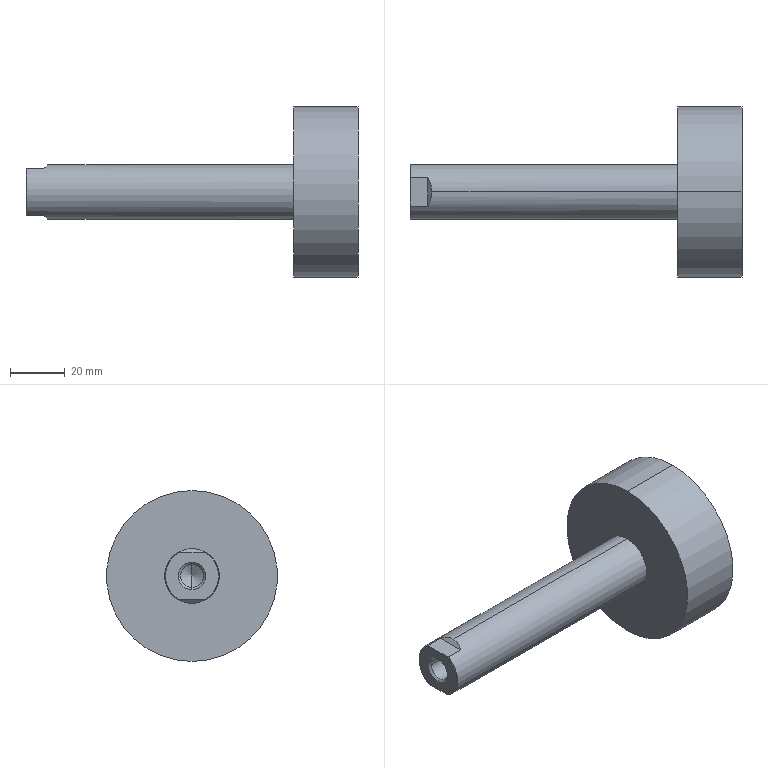Part | SolidWorks | features BaseBody 1 | 1 solid | 19 faces | box 121.5 x 62.5 x 62.5 mm | volume 101686 mm3 | plane 7 | cylinder 6 | cone 6 | commonest cylinder face diameters 8.376 x2 20 x2 62.5 x2
STEP:
#1=CARTESIAN_POINT('',(-1.5,5.268,8.5));
#2=VERTEX_POINT('',#1);
#3=CARTESIAN_POINT('',(0.,0.,10.));
#4=VERTEX_POINT('',#3);
#5=CARTESIAN_POINT('',(-1.5,5.268,8.5));
#6=CARTESIAN_POINT('',(-0.5131,3.675,9.487));
#7=CARTESIAN_POINT('',(0.,1.873,10.));
#8=CARTESIAN_POINT('',(0.,0.,10.));
#9=(BOUNDED_CURVE()B_SPLINE_CURVE(3,(#5,#6,#7,#8),.UNSPECIFIED.,.F.,.T.)B_SPLINE_CURVE_WITH_KNOTS((4,4),(5.728,6.283),.UNSPECIFIED.)CURVE()GEOMETRIC_REPRESENTATION_ITEM()RATIONAL_B_SPLINE_CURVE((1.,0.9745,0.9745,1.))REPRESENTATION_ITEM(''));
#10=EDGE_CURVE('',#2,#4,#9,.T.);
#11=ORIENTED_EDGE('',*,*,#10,.T.);
#12=CARTESIAN_POINT('',(90.,0.,10.));
#13=VERTEX_POINT('',#12);
#14=CARTESIAN_POINT('',(0.,0.,10.));
#15=DIRECTION('',(1.,0.,0.));
#16=VECTOR('',#15,1000.);
#17=LINE('',#14,#16);
#18=EDGE_CURVE('',#4,#13,#17,.T.);
#19=ORIENTED_EDGE('',*,*,#18,.T.);
#20=CARTESIAN_POINT('',(90.,0.,-10.));
#21=VERTEX_POINT('',#20);
#22=CARTESIAN_POINT('',(90.,0.,0.));
#23=DIRECTION('',(-1.,0.,0.));
#24=DIRECTION('',(0.,0.,-1.));
#25=AXIS2_PLACEMENT_3D('',#22,#23,#24);
#26=CIRCLE('',#25,10.);
#27=EDGE_CURVE('',#13,#21,#26,.T.);
#28=ORIENTED_EDGE('',*,*,#27,.T.);
#29=CARTESIAN_POINT('',(0.,0.,-10.));
#30=VERTEX_POINT('',#29);
#31=CARTESIAN_POINT('',(0.,0.,-10.));
#32=DIRECTION('',(1.,0.,0.));
#33=VECTOR('',#32,1000.);
#34=LINE('',#31,#33);
#35=EDGE_CURVE('',#30,#21,#34,.T.);
#36=ORIENTED_EDGE('',*,*,#35,.F.);
#37=CARTESIAN_POINT('',(-1.5,5.268,-8.5));
#38=VERTEX_POINT('',#37);
#39=CARTESIAN_POINT('',(0.,0.,-10.));
#40=CARTESIAN_POINT('',(0.,1.873,-10.));
#41=CARTESIAN_POINT('',(-0.5131,3.675,-9.487));
#42=CARTESIAN_POINT('',(-1.5,5.268,-8.5));
#43=(BOUNDED_CURVE()B_SPLINE_CURVE(3,(#39,#40,#41,#42),.UNSPECIFIED.,.F.,.T.)B_SPLINE_CURVE_WITH_KNOTS((4,4),(0.,0.5548),.UNSPECIFIED.)CURVE()GEOMETRIC_REPRESENTATION_ITEM()RATIONAL_B_SPLINE_CURVE((1.,0.9745,0.9745,1.))REPRESENTATION_ITEM(''));
#44=EDGE_CURVE('',#30,#38,#43,.T.);
#45=ORIENTED_EDGE('',*,*,#44,.T.);
#46=CARTESIAN_POINT('',(-7.75,5.268,-8.5));
#47=VERTEX_POINT('',#46);
#48=CARTESIAN_POINT('',(0.,5.268,-8.5));
#49=DIRECTION('',(-1.,0.,0.));
#50=VECTOR('',#49,1000.);
#51=LINE('',#48,#50);
#52=EDGE_CURVE('',#38,#47,#51,.T.);
#53=ORIENTED_EDGE('',*,*,#52,.T.);
#54=CARTESIAN_POINT('',(-7.75,5.268,8.5));
#55=VERTEX_POINT('',#54);
#56=CARTESIAN_POINT('',(-7.75,0.,0.));
#57=DIRECTION('',(1.,0.,0.));
#58=DIRECTION('',(0.,0.,-1.));
#59=AXIS2_PLACEMENT_3D('',#56,#57,#58);
#60=CIRCLE('',#59,10.);
#61=EDGE_CURVE('',#47,#55,#60,.T.);
#62=ORIENTED_EDGE('',*,*,#61,.T.);
#63=CARTESIAN_POINT('',(0.,5.268,8.5));
#64=DIRECTION('',(1.,0.,0.));
#65=VECTOR('',#64,1000.);
#66=LINE('',#63,#65);
#67=EDGE_CURVE('',#55,#2,#66,.T.);
#68=ORIENTED_EDGE('',*,*,#67,.T.);
#69=EDGE_LOOP('',(#11,#19,#28,#36,#45,#53,#62,#68));
#70=FACE_OUTER_BOUND('',#69,.T.);
#71=CARTESIAN_POINT('',(0.,0.,0.));
#72=DIRECTION('',(1.,0.,0.));
#73=DIRECTION('',(0.,0.,-1.));
#74=AXIS2_PLACEMENT_3D('',#71,#72,#73);
#75=CYLINDRICAL_SURFACE('',#74,10.);
#76=ADVANCED_FACE('',(#70),#75,.T.);
#77=CARTESIAN_POINT('',(90.,0.,-31.25));
#78=VERTEX_POINT('',#77);
#79=CARTESIAN_POINT('',(90.,0.,31.25));
#80=VERTEX_POINT('',#79);
#81=CARTESIAN_POINT('',(90.,0.,0.));
#82=DIRECTION('',(1.,0.,0.));
#83=DIRECTION('',(0.,0.,-1.));
#84=AXIS2_PLACEMENT_3D('',#81,#82,#83);
#85=CIRCLE('',#84,31.25);
#86=EDGE_CURVE('',#78,#80,#85,.T.);
#87=ORIENTED_EDGE('',*,*,#86,.T.);
#88=CARTESIAN_POINT('',(113.5,0.,31.25));
#89=VERTEX_POINT('',#88);
#90=CARTESIAN_POINT('',(113.5,0.,31.25));
#91=DIRECTION('',(1.,0.,0.));
#92=VECTOR('',#91,1000.);
#93=LINE('',#90,#92);
#94=EDGE_CURVE('',#80,#89,#93,.T.);
#95=ORIENTED_EDGE('',*,*,#94,.T.);
#96=CARTESIAN_POINT('',(113.5,0.,-31.25));
#97=VERTEX_POINT('',#96);
#98=CARTESIAN_POINT('',(113.5,0.,0.));
#99=DIRECTION('',(-1.,0.,0.));
#100=DIRECTION('',(0.,0.,-1.));
#101=AXIS2_PLACEMENT_3D('',#98,#99,#100);
#102=CIRCLE('',#101,31.25);
#103=EDGE_CURVE('',#89,#97,#102,.T.);
#104=ORIENTED_EDGE('',*,*,#103,.T.);
#105=CARTESIAN_POINT('',(113.5,0.,-31.25));
#106=DIRECTION('',(1.,0.,0.));
#107=VECTOR('',#106,1000.);
#108=LINE('',#105,#107);
#109=EDGE_CURVE('',#78,#97,#108,.T.);
#110=ORIENTED_EDGE('',*,*,#109,.F.);
#111=EDGE_LOOP('',(#87,#95,#104,#110));
#112=FACE_OUTER_BOUND('',#111,.T.);
#113=CARTESIAN_POINT('',(113.5,0.,0.));
#114=DIRECTION('',(1.,0.,0.));
#115=DIRECTION('',(0.,0.,-1.));
#116=AXIS2_PLACEMENT_3D('',#113,#114,#115);
#117=CYLINDRICAL_SURFACE('',#116,31.25);
#118=ADVANCED_FACE('',(#112),#117,.T.);
#119=CARTESIAN_POINT('',(-7.188,0.,-4.188));
#120=VERTEX_POINT('',#119);
#121=CARTESIAN_POINT('',(-7.188,-4.188,0.));
#122=VERTEX_POINT('',#121);
#123=CARTESIAN_POINT('',(-7.188,0.,0.));
#124=DIRECTION('',(-1.,0.,0.));
#125=DIRECTION('',(0.,-1.,0.));
#126=AXIS2_PLACEMENT_3D('',#123,#124,#125);
#127=CIRCLE('',#126,4.188);
#128=EDGE_CURVE('',#120,#122,#127,.T.);
#129=ORIENTED_EDGE('',*,*,#128,.F.);
#130=CARTESIAN_POINT('',(-8.,0.,-5.));
#131=VERTEX_POINT('',#130);
#132=CARTESIAN_POINT('',(-8.,0.,-5.));
#133=DIRECTION('',(-0.7071,0.,-0.7071));
#134=VECTOR('',#133,1000.);
#135=LINE('',#132,#134);
#136=EDGE_CURVE('',#120,#131,#135,.T.);
#137=ORIENTED_EDGE('',*,*,#136,.T.);
#138=CARTESIAN_POINT('',(-8.,0.,5.));
#139=VERTEX_POINT('',#138);
#140=CARTESIAN_POINT('',(-8.,0.,0.));
#141=DIRECTION('',(-1.,0.,0.));
#142=DIRECTION('',(0.,0.,1.));
#143=AXIS2_PLACEMENT_3D('',#140,#141,#142);
#144=CIRCLE('',#143,5.);
#145=EDGE_CURVE('',#131,#139,#144,.T.);
#146=ORIENTED_EDGE('',*,*,#145,.T.);
#147=CARTESIAN_POINT('',(-7.188,0.,4.188));
#148=VERTEX_POINT('',#147);
#149=CARTESIAN_POINT('',(-8.,0.,5.));
#150=DIRECTION('',(-0.7071,0.,0.7071));
#151=VECTOR('',#150,1000.);
#152=LINE('',#149,#151);
#153=EDGE_CURVE('',#148,#139,#152,.T.);
#154=ORIENTED_EDGE('',*,*,#153,.F.);
#155=CARTESIAN_POINT('',(-7.188,0.,0.));
#156=DIRECTION('',(-1.,0.,0.));
#157=DIRECTION('',(0.,-1.,0.));
#158=AXIS2_PLACEMENT_3D('',#155,#156,#157);
#159=CIRCLE('',#158,4.188);
#160=EDGE_CURVE('',#122,#148,#159,.T.);
#161=ORIENTED_EDGE('',*,*,#160,.F.);
#162=EDGE_LOOP('',(#129,#137,#146,#154,#161));
#163=FACE_OUTER_BOUND('',#162,.T.);
#164=CARTESIAN_POINT('',(-8.,0.,0.));
#165=DIRECTION('',(-1.,0.,0.));
#166=DIRECTION('',(0.,0.,1.));
#167=AXIS2_PLACEMENT_3D('',#164,#165,#166);
#168=CONICAL_SURFACE('',#167,5.,0.7854);
#169=ADVANCED_FACE('',(#163),#168,.F.);
#170=CARTESIAN_POINT('',(-7.188,4.188,0.));
#171=VERTEX_POINT('',#170);
#172=CARTESIAN_POINT('',(-7.188,0.,0.));
#173=DIRECTION('',(-1.,0.,0.));
#174=DIRECTION('',(0.,-1.,0.));
#175=AXIS2_PLACEMENT_3D('',#172,#173,#174);
#176=CIRCLE('',#175,4.188);
#177=EDGE_CURVE('',#171,#120,#176,.T.);
#178=ORIENTED_EDGE('',*,*,#177,.T.);
#179=ORIENTED_EDGE('',*,*,#128,.T.);
#180=CARTESIAN_POINT('',(10.,-4.188,0.));
#181=VERTEX_POINT('',#180);
#182=CARTESIAN_POINT('',(12.418,-4.188,0.));
#183=DIRECTION('',(1.,0.,0.));
#184=VECTOR('',#183,1000.);
#185=LINE('',#182,#184);
#186=EDGE_CURVE('',#122,#181,#185,.T.);
#187=ORIENTED_EDGE('',*,*,#186,.T.);
#188=CARTESIAN_POINT('',(10.,0.,-4.188));
#189=VERTEX_POINT('',#188);
#190=CARTESIAN_POINT('',(10.,0.,0.));
#191=DIRECTION('',(-1.,0.,0.));
#192=DIRECTION('',(0.,1.,0.));
#193=AXIS2_PLACEMENT_3D('',#190,#191,#192);
#194=CIRCLE('',#193,4.188);
#195=EDGE_CURVE('',#189,#181,#194,.T.);
#196=ORIENTED_EDGE('',*,*,#195,.F.);
#197=CARTESIAN_POINT('',(10.,4.188,0.));
#198=VERTEX_POINT('',#197);
#199=CARTESIAN_POINT('',(10.,0.,0.));
#200=DIRECTION('',(-1.,0.,0.));
#201=DIRECTION('',(0.,1.,0.));
#202=AXIS2_PLACEMENT_3D('',#199,#200,#201);
#203=CIRCLE('',#202,4.188);
#204=EDGE_CURVE('',#198,#189,#203,.T.);
#205=ORIENTED_EDGE('',*,*,#204,.F.);
#206=CARTESIAN_POINT('',(12.418,4.188,0.));
#207=DIRECTION('',(1.,0.,0.));
#208=VECTOR('',#207,1000.);
#209=LINE('',#206,#208);
#210=EDGE_CURVE('',#171,#198,#209,.T.);
#211=ORIENTED_EDGE('',*,*,#210,.F.);
#212=EDGE_LOOP('',(#178,#179,#187,#196,#205,#211));
#213=FACE_OUTER_BOUND('',#212,.T.);
#214=CARTESIAN_POINT('',(12.418,0.,0.));
#215=DIRECTION('',(1.,0.,0.));
#216=DIRECTION('',(0.,1.,0.));
#217=AXIS2_PLACEMENT_3D('',#214,#215,#216);
#218=CYLINDRICAL_SURFACE('',#217,4.188);
#219=ADVANCED_FACE('',(#213),#218,.F.);
#220=CARTESIAN_POINT('',(12.418,0.,0.));
#221=VERTEX_POINT('',#220);
#222=CARTESIAN_POINT('',(10.,0.,4.188));
#223=VERTEX_POINT('',#222);
#224=CARTESIAN_POINT('',(10.,0.,4.188));
#225=DIRECTION('',(-0.5,0.,0.866));
#226=VECTOR('',#225,1000.);
#227=LINE('',#224,#226);
#228=EDGE_CURVE('',#221,#223,#227,.T.);
#229=ORIENTED_EDGE('',*,*,#228,.F.);
#230=CARTESIAN_POINT('',(10.,0.,-4.188));
#231=DIRECTION('',(-0.5,0.,-0.866));
#232=VECTOR('',#231,1000.);
#233=LINE('',#230,#232);
#234=EDGE_CURVE('',#221,#189,#233,.T.);
#235=ORIENTED_EDGE('',*,*,#234,.T.);
#236=ORIENTED_EDGE('',*,*,#195,.T.);
#237=CARTESIAN_POINT('',(10.,0.,0.));
#238=DIRECTION('',(-1.,0.,0.));
#239=DIRECTION('',(0.,1.,0.));
#240=AXIS2_PLACEMENT_3D('',#237,#238,#239);
#241=CIRCLE('',#240,4.188);
#242=EDGE_CURVE('',#181,#223,#241,.T.);
#243=ORIENTED_EDGE('',*,*,#242,.T.);
#244=EDGE_LOOP('',(#229,#235,#236,#243));
#245=FACE_OUTER_BOUND('',#244,.T.);
#246=CARTESIAN_POINT('',(10.,0.,0.));
#247=DIRECTION('',(-1.,0.,0.));
#248=DIRECTION('',(0.,0.,1.));
#249=AXIS2_PLACEMENT_3D('',#246,#247,#248);
#250=CONICAL_SURFACE('',#249,4.188,1.047);
#251=ADVANCED_FACE('',(#245),#250,.F.);
#252=ORIENTED_EDGE('',*,*,#18,.F.);
#253=CARTESIAN_POINT('',(-1.5,-5.268,8.5));
#254=VERTEX_POINT('',#253);
#255=CARTESIAN_POINT('',(0.,0.,10.));
#256=CARTESIAN_POINT('',(0.,-1.873,10.));
#257=CARTESIAN_POINT('',(-0.5131,-3.675,9.487));
#258=CARTESIAN_POINT('',(-1.5,-5.268,8.5));
#259=(BOUNDED_CURVE()B_SPLINE_CURVE(3,(#255,#256,#257,#258),.UNSPECIFIED.,.F.,.T.)B_SPLINE_CURVE_WITH_KNOTS((4,4),(0.,0.5548),.UNSPECIFIED.)CURVE()GEOMETRIC_REPRESENTATION_ITEM()RATIONAL_B_SPLINE_CURVE((1.,0.9745,0.9745,1.))REPRESENTATION_ITEM(''));
#260=EDGE_CURVE('',#4,#254,#259,.T.);
#261=ORIENTED_EDGE('',*,*,#260,.T.);
#262=CARTESIAN_POINT('',(-7.75,-5.268,8.5));
#263=VERTEX_POINT('',#262);
#264=CARTESIAN_POINT('',(0.,-5.268,8.5));
#265=DIRECTION('',(-1.,0.,0.));
#266=VECTOR('',#265,1000.);
#267=LINE('',#264,#266);
#268=EDGE_CURVE('',#254,#263,#267,.T.);
#269=ORIENTED_EDGE('',*,*,#268,.T.);
#270=CARTESIAN_POINT('',(-7.75,-5.268,-8.5));
#271=VERTEX_POINT('',#270);
#272=CARTESIAN_POINT('',(-7.75,0.,0.));
#273=DIRECTION('',(1.,0.,0.));
#274=DIRECTION('',(0.,0.,-1.));
#275=AXIS2_PLACEMENT_3D('',#272,#273,#274);
#276=CIRCLE('',#275,10.);
#277=EDGE_CURVE('',#263,#271,#276,.T.);
#278=ORIENTED_EDGE('',*,*,#277,.T.);
#279=CARTESIAN_POINT('',(-1.5,-5.268,-8.5));
#280=VERTEX_POINT('',#279);
#281=CARTESIAN_POINT('',(0.,-5.268,-8.5));
#282=DIRECTION('',(1.,0.,0.));
#283=VECTOR('',#282,1000.);
#284=LINE('',#281,#283);
#285=EDGE_CURVE('',#271,#280,#284,.T.);
#286=ORIENTED_EDGE('',*,*,#285,.T.);
#287=CARTESIAN_POINT('',(-1.5,-5.268,-8.5));
#288=CARTESIAN_POINT('',(-0.5131,-3.675,-9.487));
#289=CARTESIAN_POINT('',(0.,-1.873,-10.));
#290=CARTESIAN_POINT('',(0.,0.,-10.));
#291=(BOUNDED_CURVE()B_SPLINE_CURVE(3,(#287,#288,#289,#290),.UNSPECIFIED.,.F.,.T.)B_SPLINE_CURVE_WITH_KNOTS((4,4),(5.728,6.283),.UNSPECIFIED.)CURVE()GEOMETRIC_REPRESENTATION_ITEM()RATIONAL_B_SPLINE_CURVE((1.,0.9745,0.9745,1.))REPRESENTATION_ITEM(''));
#292=EDGE_CURVE('',#280,#30,#291,.T.);
#293=ORIENTED_EDGE('',*,*,#292,.T.);
#294=ORIENTED_EDGE('',*,*,#35,.T.);
#295=CARTESIAN_POINT('',(90.,0.,0.));
#296=DIRECTION('',(-1.,0.,0.));
#297=DIRECTION('',(0.,0.,-1.));
#298=AXIS2_PLACEMENT_3D('',#295,#296,#297);
#299=CIRCLE('',#298,10.);
#300=EDGE_CURVE('',#21,#13,#299,.T.);
#301=ORIENTED_EDGE('',*,*,#300,.T.);
#302=EDGE_LOOP('',(#252,#261,#269,#278,#286,#293,#294,#301));
#303=FACE_OUTER_BOUND('',#302,.T.);
#304=CARTESIAN_POINT('',(0.,0.,0.));
#305=DIRECTION('',(1.,0.,0.));
#306=DIRECTION('',(0.,0.,-1.));
#307=AXIS2_PLACEMENT_3D('',#304,#305,#306);
#308=CYLINDRICAL_SURFACE('',#307,10.);
#309=ADVANCED_FACE('',(#303),#308,.T.);
#310=ORIENTED_EDGE('',*,*,#10,.F.);
#311=CARTESIAN_POINT('',(-1.5,17.,8.5));
#312=DIRECTION('',(0.,-1.,0.));
#313=VECTOR('',#312,1000.);
#314=LINE('',#311,#313);
#315=EDGE_CURVE('',#2,#254,#314,.T.);
#316=ORIENTED_EDGE('',*,*,#315,.T.);
#317=ORIENTED_EDGE('',*,*,#260,.F.);
#318=EDGE_LOOP('',(#310,#316,#317));
#319=FACE_OUTER_BOUND('',#318,.T.);
#320=CARTESIAN_POINT('',(3.5,17.,13.5));
#321=DIRECTION('',(-0.7071,0.,0.7071));
#322=DIRECTION('',(0.7071,0.,0.7071));
#323=AXIS2_PLACEMENT_3D('',#320,#321,#322);
#324=PLANE('',#323);
#325=ADVANCED_FACE('',(#319),#324,.T.);
#326=CARTESIAN_POINT('',(-8.,4.776,8.5));
#327=VERTEX_POINT('',#326);
#328=CARTESIAN_POINT('',(-7.75,5.268,8.5));
#329=CARTESIAN_POINT('',(-7.837,5.102,8.5));
#330=CARTESIAN_POINT('',(-7.921,4.938,8.5));
#331=CARTESIAN_POINT('',(-8.,4.776,8.5));
#332=B_SPLINE_CURVE_WITH_KNOTS('',3,(#328,#329,#330,#331),.UNSPECIFIED.,.F.,.F.,(4,4),(0.,1.),.UNSPECIFIED.);
#333=EDGE_CURVE('',#55,#327,#332,.T.);
#334=ORIENTED_EDGE('',*,*,#333,.T.);
#335=CARTESIAN_POINT('',(-8.,-4.776,8.5));
#336=VERTEX_POINT('',#335);
#337=CARTESIAN_POINT('',(-8.,17.,8.5));
#338=DIRECTION('',(0.,-1.,0.));
#339=VECTOR('',#338,1000.);
#340=LINE('',#337,#339);
#341=EDGE_CURVE('',#327,#336,#340,.T.);
#342=ORIENTED_EDGE('',*,*,#341,.T.);
#343=CARTESIAN_POINT('',(-8.,-4.776,8.5));
#344=CARTESIAN_POINT('',(-7.921,-4.938,8.5));
#345=CARTESIAN_POINT('',(-7.837,-5.102,8.5));
#346=CARTESIAN_POINT('',(-7.75,-5.268,8.5));
#347=B_SPLINE_CURVE_WITH_KNOTS('',3,(#343,#344,#345,#346),.UNSPECIFIED.,.F.,.F.,(4,4),(0.,1.),.UNSPECIFIED.);
#348=EDGE_CURVE('',#336,#263,#347,.T.);
#349=ORIENTED_EDGE('',*,*,#348,.T.);
#350=ORIENTED_EDGE('',*,*,#268,.F.);
#351=ORIENTED_EDGE('',*,*,#315,.F.);
#352=ORIENTED_EDGE('',*,*,#67,.F.);
#353=EDGE_LOOP('',(#334,#342,#349,#350,#351,#352));
#354=FACE_OUTER_BOUND('',#353,.T.);
#355=CARTESIAN_POINT('',(-1.5,17.,8.5));
#356=DIRECTION('',(0.,0.,1.));
#357=DIRECTION('',(1.,0.,0.));
#358=AXIS2_PLACEMENT_3D('',#355,#356,#357);
#359=PLANE('',#358);
#360=ADVANCED_FACE('',(#354),#359,.T.);
#361=ORIENTED_EDGE('',*,*,#333,.F.);
#362=ORIENTED_EDGE('',*,*,#61,.F.);
#363=CARTESIAN_POINT('',(-8.,4.776,-8.5));
#364=VERTEX_POINT('',#363);
#365=CARTESIAN_POINT('',(-7.75,5.268,-8.5));
#366=CARTESIAN_POINT('',(-7.837,5.103,-8.5));
#367=CARTESIAN_POINT('',(-7.92,4.939,-8.5));
#368=CARTESIAN_POINT('',(-8.,4.776,-8.5));
#369=B_SPLINE_CURVE_WITH_KNOTS('',3,(#365,#366,#367,#368),.UNSPECIFIED.,.F.,.F.,(4,4),(0.,1.),.UNSPECIFIED.);
#370=EDGE_CURVE('',#47,#364,#369,.T.);
#371=ORIENTED_EDGE('',*,*,#370,.T.);
#372=CARTESIAN_POINT('',(-8.,0.,0.));
#373=DIRECTION('',(1.,0.,0.));
#374=DIRECTION('',(0.,0.,-1.));
#375=AXIS2_PLACEMENT_3D('',#372,#373,#374);
#376=CIRCLE('',#375,9.75);
#377=EDGE_CURVE('',#364,#327,#376,.T.);
#378=ORIENTED_EDGE('',*,*,#377,.T.);
#379=EDGE_LOOP('',(#361,#362,#371,#378));
#380=FACE_OUTER_BOUND('',#379,.T.);
#381=CARTESIAN_POINT('',(-7.75,0.,0.));
#382=DIRECTION('',(1.,0.,0.));
#383=DIRECTION('',(0.,0.,-1.));
#384=AXIS2_PLACEMENT_3D('',#381,#382,#383);
#385=CONICAL_SURFACE('',#384,10.,0.7854);
#386=ADVANCED_FACE('',(#380),#385,.T.);
#387=CARTESIAN_POINT('',(-8.,-4.776,-8.5));
#388=VERTEX_POINT('',#387);
#389=CARTESIAN_POINT('',(-7.75,-5.268,-8.5));
#390=CARTESIAN_POINT('',(-7.837,-5.102,-8.5));
#391=CARTESIAN_POINT('',(-7.921,-4.938,-8.5));
#392=CARTESIAN_POINT('',(-8.,-4.776,-8.5));
#393=B_SPLINE_CURVE_WITH_KNOTS('',3,(#389,#390,#391,#392),.UNSPECIFIED.,.F.,.F.,(4,4),(0.,1.),.UNSPECIFIED.);
#394=EDGE_CURVE('',#271,#388,#393,.T.);
#395=ORIENTED_EDGE('',*,*,#394,.T.);
#396=CARTESIAN_POINT('',(-8.,17.,-8.5));
#397=DIRECTION('',(0.,1.,0.));
#398=VECTOR('',#397,1000.);
#399=LINE('',#396,#398);
#400=EDGE_CURVE('',#388,#364,#399,.T.);
#401=ORIENTED_EDGE('',*,*,#400,.T.);
#402=ORIENTED_EDGE('',*,*,#370,.F.);
#403=ORIENTED_EDGE('',*,*,#52,.F.);
#404=CARTESIAN_POINT('',(-1.5,17.,-8.5));
#405=DIRECTION('',(0.,-1.,0.));
#406=VECTOR('',#405,1000.);
#407=LINE('',#404,#406);
#408=EDGE_CURVE('',#38,#280,#407,.T.);
#409=ORIENTED_EDGE('',*,*,#408,.T.);
#410=ORIENTED_EDGE('',*,*,#285,.F.);
#411=EDGE_LOOP('',(#395,#401,#402,#403,#409,#410));
#412=FACE_OUTER_BOUND('',#411,.T.);
#413=CARTESIAN_POINT('',(-8.,17.,-8.5));
#414=DIRECTION('',(0.,0.,-1.));
#415=DIRECTION('',(-1.,0.,0.));
#416=AXIS2_PLACEMENT_3D('',#413,#414,#415);
#417=PLANE('',#416);
#418=ADVANCED_FACE('',(#412),#417,.T.);
#419=ORIENTED_EDGE('',*,*,#292,.F.);
#420=ORIENTED_EDGE('',*,*,#408,.F.);
#421=ORIENTED_EDGE('',*,*,#44,.F.);
#422=EDGE_LOOP('',(#419,#420,#421));
#423=FACE_OUTER_BOUND('',#422,.T.);
#424=CARTESIAN_POINT('',(-1.5,17.,-8.5));
#425=DIRECTION('',(-0.7071,0.,-0.7071));
#426=DIRECTION('',(-0.7071,0.,0.7071));
#427=AXIS2_PLACEMENT_3D('',#424,#425,#426);
#428=PLANE('',#427);
#429=ADVANCED_FACE('',(#423),#428,.T.);
#430=ORIENTED_EDGE('',*,*,#394,.F.);
#431=ORIENTED_EDGE('',*,*,#277,.F.);
#432=ORIENTED_EDGE('',*,*,#348,.F.);
#433=CARTESIAN_POINT('',(-8.,0.,0.));
#434=DIRECTION('',(1.,0.,0.));
#435=DIRECTION('',(0.,0.,-1.));
#436=AXIS2_PLACEMENT_3D('',#433,#434,#435);
#437=CIRCLE('',#436,9.75);
#438=EDGE_CURVE('',#336,#388,#437,.T.);
#439=ORIENTED_EDGE('',*,*,#438,.T.);
#440=EDGE_LOOP('',(#430,#431,#432,#439));
#441=FACE_OUTER_BOUND('',#440,.T.);
#442=CARTESIAN_POINT('',(-7.75,0.,0.));
#443=DIRECTION('',(1.,0.,0.));
#444=DIRECTION('',(0.,0.,-1.));
#445=AXIS2_PLACEMENT_3D('',#442,#443,#444);
#446=CONICAL_SURFACE('',#445,10.,0.7854);
#447=ADVANCED_FACE('',(#441),#446,.T.);
#448=ORIENTED_EDGE('',*,*,#300,.F.);
#449=ORIENTED_EDGE('',*,*,#27,.F.);
#450=EDGE_LOOP('',(#448,#449));
#451=FACE_BOUND('',#450,.T.);
#452=ORIENTED_EDGE('',*,*,#86,.F.);
#453=CARTESIAN_POINT('',(90.,0.,0.));
#454=DIRECTION('',(1.,0.,0.));
#455=DIRECTION('',(0.,0.,-1.));
#456=AXIS2_PLACEMENT_3D('',#453,#454,#455);
#457=CIRCLE('',#456,31.25);
#458=EDGE_CURVE('',#80,#78,#457,.T.);
#459=ORIENTED_EDGE('',*,*,#458,.F.);
#460=EDGE_LOOP('',(#452,#459));
#461=FACE_OUTER_BOUND('',#460,.T.);
#462=CARTESIAN_POINT('',(90.,10.,0.));
#463=DIRECTION('',(1.,0.,0.));
#464=DIRECTION('',(0.,0.,-1.));
#465=AXIS2_PLACEMENT_3D('',#462,#463,#464);
#466=PLANE('',#465);
#467=ADVANCED_FACE('',(#451,#461),#466,.F.);
#468=CARTESIAN_POINT('',(-8.,0.,0.));
#469=DIRECTION('',(-1.,0.,0.));
#470=DIRECTION('',(0.,0.,1.));
#471=AXIS2_PLACEMENT_3D('',#468,#469,#470);
#472=CIRCLE('',#471,5.);
#473=EDGE_CURVE('',#139,#131,#472,.T.);
#474=ORIENTED_EDGE('',*,*,#473,.F.);
#475=ORIENTED_EDGE('',*,*,#145,.F.);
#476=EDGE_LOOP('',(#474,#475));
#477=FACE_BOUND('',#476,.T.);
#478=ORIENTED_EDGE('',*,*,#400,.F.);
#479=ORIENTED_EDGE('',*,*,#438,.F.);
#480=ORIENTED_EDGE('',*,*,#341,.F.);
#481=ORIENTED_EDGE('',*,*,#377,.F.);
#482=EDGE_LOOP('',(#478,#479,#480,#481));
#483=FACE_OUTER_BOUND('',#482,.T.);
#484=CARTESIAN_POINT('',(-8.,0.,0.));
#485=DIRECTION('',(1.,0.,0.));
#486=DIRECTION('',(0.,0.,-1.));
#487=AXIS2_PLACEMENT_3D('',#484,#485,#486);
#488=PLANE('',#487);
#489=ADVANCED_FACE('',(#477,#483),#488,.F.);
#490=ORIENTED_EDGE('',*,*,#94,.F.);
#491=ORIENTED_EDGE('',*,*,#458,.T.);
#492=ORIENTED_EDGE('',*,*,#109,.T.);
#493=CARTESIAN_POINT('',(113.5,0.,0.));
#494=DIRECTION('',(-1.,0.,0.));
#495=DIRECTION('',(0.,0.,-1.));
#496=AXIS2_PLACEMENT_3D('',#493,#494,#495);
#497=CIRCLE('',#496,31.25);
#498=EDGE_CURVE('',#97,#89,#497,.T.);
#499=ORIENTED_EDGE('',*,*,#498,.T.);
#500=EDGE_LOOP('',(#490,#491,#492,#499));
#501=FACE_OUTER_BOUND('',#500,.T.);
#502=CARTESIAN_POINT('',(113.5,0.,0.));
#503=DIRECTION('',(1.,0.,0.));
#504=DIRECTION('',(0.,0.,-1.));
#505=AXIS2_PLACEMENT_3D('',#502,#503,#504);
#506=CYLINDRICAL_SURFACE('',#505,31.25);
#507=ADVANCED_FACE('',(#501),#506,.T.);
#508=ORIENTED_EDGE('',*,*,#136,.F.);
#509=ORIENTED_EDGE('',*,*,#177,.F.);
#510=CARTESIAN_POINT('',(-7.188,0.,0.));
#511=DIRECTION('',(-1.,0.,0.));
#512=DIRECTION('',(0.,-1.,0.));
#513=AXIS2_PLACEMENT_3D('',#510,#511,#512);
#514=CIRCLE('',#513,4.188);
#515=EDGE_CURVE('',#148,#171,#514,.T.);
#516=ORIENTED_EDGE('',*,*,#515,.F.);
#517=ORIENTED_EDGE('',*,*,#153,.T.);
#518=ORIENTED_EDGE('',*,*,#473,.T.);
#519=EDGE_LOOP('',(#508,#509,#516,#517,#518));
#520=FACE_OUTER_BOUND('',#519,.T.);
#521=CARTESIAN_POINT('',(-8.,0.,0.));
#522=DIRECTION('',(-1.,0.,0.));
#523=DIRECTION('',(0.,0.,1.));
#524=AXIS2_PLACEMENT_3D('',#521,#522,#523);
#525=CONICAL_SURFACE('',#524,5.,0.7854);
#526=ADVANCED_FACE('',(#520),#525,.F.);
#527=ORIENTED_EDGE('',*,*,#498,.F.);
#528=ORIENTED_EDGE('',*,*,#103,.F.);
#529=EDGE_LOOP('',(#527,#528));
#530=FACE_OUTER_BOUND('',#529,.T.);
#531=CARTESIAN_POINT('',(113.5,31.25,0.));
#532=DIRECTION('',(-1.,0.,0.));
#533=DIRECTION('',(0.,0.,1.));
#534=AXIS2_PLACEMENT_3D('',#531,#532,#533);
#535=PLANE('',#534);
#536=ADVANCED_FACE('',(#530),#535,.F.);
#537=ORIENTED_EDGE('',*,*,#186,.F.);
#538=ORIENTED_EDGE('',*,*,#160,.T.);
#539=ORIENTED_EDGE('',*,*,#515,.T.);
#540=ORIENTED_EDGE('',*,*,#210,.T.);
#541=CARTESIAN_POINT('',(10.,0.,0.));
#542=DIRECTION('',(-1.,0.,0.));
#543=DIRECTION('',(0.,1.,0.));
#544=AXIS2_PLACEMENT_3D('',#541,#542,#543);
#545=CIRCLE('',#544,4.188);
#546=EDGE_CURVE('',#223,#198,#545,.T.);
#547=ORIENTED_EDGE('',*,*,#546,.F.);
#548=ORIENTED_EDGE('',*,*,#242,.F.);
#549=EDGE_LOOP('',(#537,#538,#539,#540,#547,#548));
#550=FACE_OUTER_BOUND('',#549,.T.);
#551=CARTESIAN_POINT('',(12.418,0.,0.));
#552=DIRECTION('',(1.,0.,0.));
#553=DIRECTION('',(0.,1.,0.));
#554=AXIS2_PLACEMENT_3D('',#551,#552,#553);
#555=CYLINDRICAL_SURFACE('',#554,4.188);
#556=ADVANCED_FACE('',(#550),#555,.F.);
#557=ORIENTED_EDGE('',*,*,#234,.F.);
#558=ORIENTED_EDGE('',*,*,#228,.T.);
#559=ORIENTED_EDGE('',*,*,#546,.T.);
#560=ORIENTED_EDGE('',*,*,#204,.T.);
#561=EDGE_LOOP('',(#557,#558,#559,#560));
#562=FACE_OUTER_BOUND('',#561,.T.);
#563=CARTESIAN_POINT('',(10.,0.,0.));
#564=DIRECTION('',(-1.,0.,0.));
#565=DIRECTION('',(0.,0.,1.));
#566=AXIS2_PLACEMENT_3D('',#563,#564,#565);
#567=CONICAL_SURFACE('',#566,4.188,1.047);
#568=ADVANCED_FACE('',(#562),#567,.F.);
#569=CLOSED_SHELL('',(#76,#118,#169,#219,#251,#309,#325,#360,#386,#418,#429,#447,#467,#489,#507,#526,#536,#556,#568));
#570=MANIFOLD_SOLID_BREP('',#569);
#571=CARTESIAN_POINT('',(0.,0.,0.));
#572=DIRECTION('',(0.,0.,1.));
#573=DIRECTION('',(1.,0.,0.));
#574=AXIS2_PLACEMENT_3D('',#571,#572,#573);
#575=(LENGTH_UNIT()NAMED_UNIT(*)SI_UNIT(.MILLI.,.METRE.));
#576=UNCERTAINTY_MEASURE_WITH_UNIT(LENGTH_MEASURE(0.00001),#575,'','');
#577=(NAMED_UNIT(*)PLANE_ANGLE_UNIT()SI_UNIT($,.RADIAN.));
#578=(NAMED_UNIT(*)SI_UNIT($,.STERADIAN.)SOLID_ANGLE_UNIT());
#579=(GEOMETRIC_REPRESENTATION_CONTEXT(3)GLOBAL_UNCERTAINTY_ASSIGNED_CONTEXT((#576))GLOBAL_UNIT_ASSIGNED_CONTEXT((#575,#577,#578))REPRESENTATION_CONTEXT('',''));
#580=ADVANCED_BREP_SHAPE_REPRESENTATION('',(#570,#574),#579);